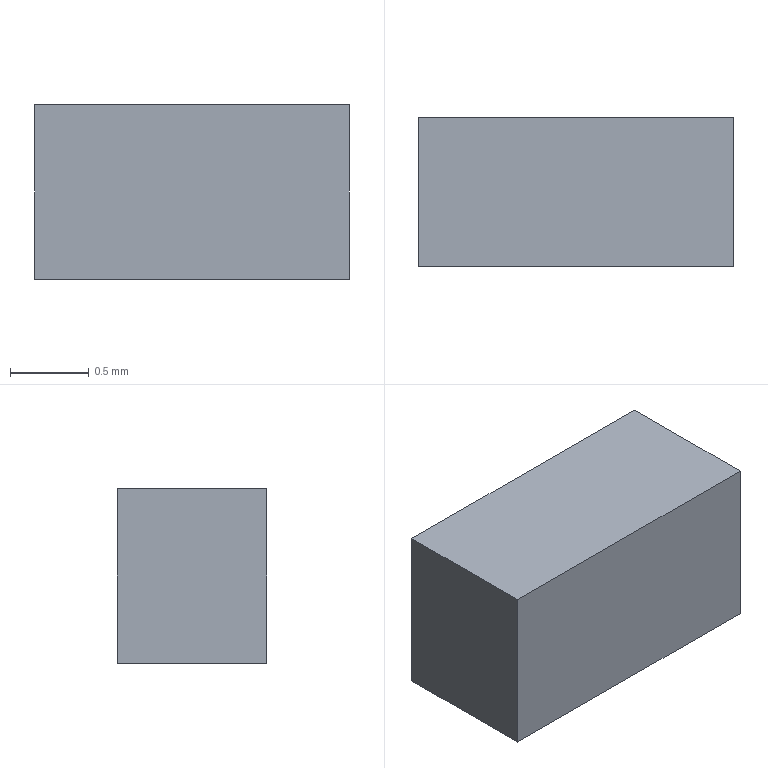Part | Creo | 1 solid | 6 faces | box 2 x 0.95 x 1.107 mm | volume 2.103 mm3 | plane 6
STEP:
#1=CARTESIAN_POINT('',(0.,0.,0.));
#2=DIRECTION('',(0.,0.,1.));
#3=DIRECTION('',(1.,0.,0.));
#4=AXIS2_PLACEMENT_3D('',#1,#2,#3);
#5=CARTESIAN_POINT('',(-1.,-0.475,0.));
#6=VERTEX_POINT('',#5);
#7=CARTESIAN_POINT('',(1.,-0.475,0.));
#8=VERTEX_POINT('',#7);
#9=CARTESIAN_POINT('',(-1.,-0.475,0.));
#10=DIRECTION('',(1.,0.,0.));
#11=VECTOR('',#10,2.);
#12=LINE('',#9,#11);
#13=EDGE_CURVE('',#6,#8,#12,.T.);
#14=ORIENTED_EDGE('',*,*,#13,.T.);
#15=CARTESIAN_POINT('',(1.,0.475,0.));
#16=VERTEX_POINT('',#15);
#17=CARTESIAN_POINT('',(1.,-0.475,0.));
#18=DIRECTION('',(0.,1.,0.));
#19=VECTOR('',#18,0.95);
#20=LINE('',#17,#19);
#21=EDGE_CURVE('',#8,#16,#20,.T.);
#22=ORIENTED_EDGE('',*,*,#21,.T.);
#23=CARTESIAN_POINT('',(-1.,0.475,0.));
#24=VERTEX_POINT('',#23);
#25=CARTESIAN_POINT('',(1.,0.475,0.));
#26=DIRECTION('',(-1.,0.,0.));
#27=VECTOR('',#26,2.);
#28=LINE('',#25,#27);
#29=EDGE_CURVE('',#16,#24,#28,.T.);
#30=ORIENTED_EDGE('',*,*,#29,.T.);
#31=CARTESIAN_POINT('',(-1.,0.475,0.));
#32=DIRECTION('',(0.,-1.,0.));
#33=VECTOR('',#32,0.95);
#34=LINE('',#31,#33);
#35=EDGE_CURVE('',#24,#6,#34,.T.);
#36=ORIENTED_EDGE('',*,*,#35,.T.);
#37=EDGE_LOOP('',(#14,#22,#30,#36));
#38=FACE_OUTER_BOUND('',#37,.F.);
#39=CARTESIAN_POINT('',(0.,0.,0.));
#40=DIRECTION('',(0.,0.,1.));
#41=DIRECTION('',(1.,0.,0.));
#42=AXIS2_PLACEMENT_3D('',#39,#40,#41);
#43=PLANE('',#42);
#44=ADVANCED_FACE('',(#38),#43,.F.);
#45=ORIENTED_EDGE('',*,*,#13,.F.);
#46=CARTESIAN_POINT('',(-1.,-0.475,1.107));
#47=VERTEX_POINT('',#46);
#48=CARTESIAN_POINT('',(-1.,-0.475,0.));
#49=DIRECTION('',(0.,0.,1.));
#50=VECTOR('',#49,1.107);
#51=LINE('',#48,#50);
#52=EDGE_CURVE('',#6,#47,#51,.T.);
#53=ORIENTED_EDGE('',*,*,#52,.T.);
#54=CARTESIAN_POINT('',(1.,-0.475,1.107));
#55=VERTEX_POINT('',#54);
#56=CARTESIAN_POINT('',(-1.,-0.475,1.107));
#57=DIRECTION('',(1.,0.,0.));
#58=VECTOR('',#57,2.);
#59=LINE('',#56,#58);
#60=EDGE_CURVE('',#47,#55,#59,.T.);
#61=ORIENTED_EDGE('',*,*,#60,.T.);
#62=CARTESIAN_POINT('',(1.,-0.475,0.));
#63=DIRECTION('',(0.,0.,1.));
#64=VECTOR('',#63,1.107);
#65=LINE('',#62,#64);
#66=EDGE_CURVE('',#8,#55,#65,.T.);
#67=ORIENTED_EDGE('',*,*,#66,.F.);
#68=EDGE_LOOP('',(#45,#53,#61,#67));
#69=FACE_OUTER_BOUND('',#68,.F.);
#70=CARTESIAN_POINT('',(-1.,-0.475,0.));
#71=DIRECTION('',(0.,-1.,0.));
#72=DIRECTION('',(1.,0.,0.));
#73=AXIS2_PLACEMENT_3D('',#70,#71,#72);
#74=PLANE('',#73);
#75=ADVANCED_FACE('',(#69),#74,.T.);
#76=ORIENTED_EDGE('',*,*,#35,.F.);
#77=CARTESIAN_POINT('',(-1.,0.475,1.107));
#78=VERTEX_POINT('',#77);
#79=CARTESIAN_POINT('',(-1.,0.475,0.));
#80=DIRECTION('',(0.,0.,1.));
#81=VECTOR('',#80,1.107);
#82=LINE('',#79,#81);
#83=EDGE_CURVE('',#24,#78,#82,.T.);
#84=ORIENTED_EDGE('',*,*,#83,.T.);
#85=CARTESIAN_POINT('',(-1.,0.475,1.107));
#86=DIRECTION('',(0.,-1.,0.));
#87=VECTOR('',#86,0.95);
#88=LINE('',#85,#87);
#89=EDGE_CURVE('',#78,#47,#88,.T.);
#90=ORIENTED_EDGE('',*,*,#89,.T.);
#91=ORIENTED_EDGE('',*,*,#52,.F.);
#92=EDGE_LOOP('',(#76,#84,#90,#91));
#93=FACE_OUTER_BOUND('',#92,.F.);
#94=CARTESIAN_POINT('',(-1.,0.475,0.));
#95=DIRECTION('',(-1.,0.,0.));
#96=DIRECTION('',(0.,-1.,0.));
#97=AXIS2_PLACEMENT_3D('',#94,#95,#96);
#98=PLANE('',#97);
#99=ADVANCED_FACE('',(#93),#98,.T.);
#100=ORIENTED_EDGE('',*,*,#29,.F.);
#101=CARTESIAN_POINT('',(1.,0.475,1.107));
#102=VERTEX_POINT('',#101);
#103=CARTESIAN_POINT('',(1.,0.475,0.));
#104=DIRECTION('',(0.,0.,1.));
#105=VECTOR('',#104,1.107);
#106=LINE('',#103,#105);
#107=EDGE_CURVE('',#16,#102,#106,.T.);
#108=ORIENTED_EDGE('',*,*,#107,.T.);
#109=CARTESIAN_POINT('',(1.,0.475,1.107));
#110=DIRECTION('',(-1.,0.,0.));
#111=VECTOR('',#110,2.);
#112=LINE('',#109,#111);
#113=EDGE_CURVE('',#102,#78,#112,.T.);
#114=ORIENTED_EDGE('',*,*,#113,.T.);
#115=ORIENTED_EDGE('',*,*,#83,.F.);
#116=EDGE_LOOP('',(#100,#108,#114,#115));
#117=FACE_OUTER_BOUND('',#116,.F.);
#118=CARTESIAN_POINT('',(1.,0.475,0.));
#119=DIRECTION('',(0.,1.,0.));
#120=DIRECTION('',(-1.,0.,0.));
#121=AXIS2_PLACEMENT_3D('',#118,#119,#120);
#122=PLANE('',#121);
#123=ADVANCED_FACE('',(#117),#122,.T.);
#124=ORIENTED_EDGE('',*,*,#21,.F.);
#125=ORIENTED_EDGE('',*,*,#66,.T.);
#126=CARTESIAN_POINT('',(1.,-0.475,1.107));
#127=DIRECTION('',(0.,1.,0.));
#128=VECTOR('',#127,0.95);
#129=LINE('',#126,#128);
#130=EDGE_CURVE('',#55,#102,#129,.T.);
#131=ORIENTED_EDGE('',*,*,#130,.T.);
#132=ORIENTED_EDGE('',*,*,#107,.F.);
#133=EDGE_LOOP('',(#124,#125,#131,#132));
#134=FACE_OUTER_BOUND('',#133,.F.);
#135=CARTESIAN_POINT('',(1.,-0.475,0.));
#136=DIRECTION('',(1.,0.,0.));
#137=DIRECTION('',(0.,1.,0.));
#138=AXIS2_PLACEMENT_3D('',#135,#136,#137);
#139=PLANE('',#138);
#140=ADVANCED_FACE('',(#134),#139,.T.);
#141=ORIENTED_EDGE('',*,*,#60,.F.);
#142=ORIENTED_EDGE('',*,*,#89,.F.);
#143=ORIENTED_EDGE('',*,*,#113,.F.);
#144=ORIENTED_EDGE('',*,*,#130,.F.);
#145=EDGE_LOOP('',(#141,#142,#143,#144));
#146=FACE_OUTER_BOUND('',#145,.F.);
#147=CARTESIAN_POINT('',(0.,0.,1.107));
#148=DIRECTION('',(0.,0.,1.));
#149=DIRECTION('',(1.,0.,0.));
#150=AXIS2_PLACEMENT_3D('',#147,#148,#149);
#151=PLANE('',#150);
#152=ADVANCED_FACE('',(#146),#151,.T.);
#153=CLOSED_SHELL('',(#44,#75,#99,#123,#140,#152));
#154=MANIFOLD_SOLID_BREP('',#153);
#155=(LENGTH_UNIT()NAMED_UNIT(*)SI_UNIT(.MILLI.,.METRE.));
#156=UNCERTAINTY_MEASURE_WITH_UNIT(LENGTH_MEASURE(0.0002475),#155,'','');
#157=(NAMED_UNIT(*)PLANE_ANGLE_UNIT()SI_UNIT($,.RADIAN.));
#158=PLANE_ANGLE_MEASURE_WITH_UNIT(PLANE_ANGLE_MEASURE(0.01745),#157);
#159=(CONVERSION_BASED_UNIT('DEGREE',#158)NAMED_UNIT(*)PLANE_ANGLE_UNIT());
#160=(NAMED_UNIT(*)SI_UNIT($,.STERADIAN.)SOLID_ANGLE_UNIT());
#161=(GEOMETRIC_REPRESENTATION_CONTEXT(3)GLOBAL_UNCERTAINTY_ASSIGNED_CONTEXT((#156))GLOBAL_UNIT_ASSIGNED_CONTEXT((#155,#159,#160))REPRESENTATION_CONTEXT('',''));
#162=ADVANCED_BREP_SHAPE_REPRESENTATION('',(#4,#154),#161);